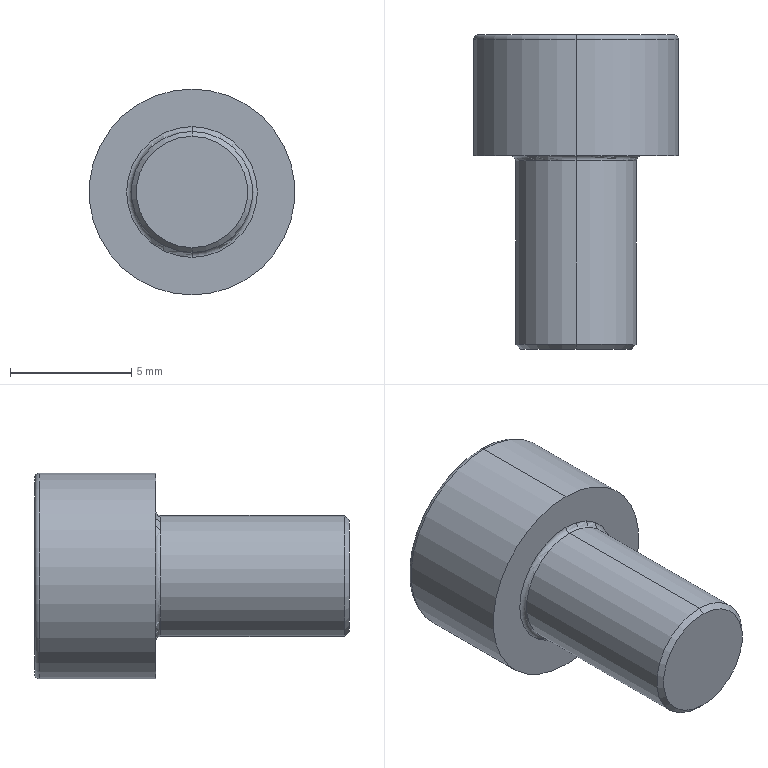Part | STEP file | 1 solid | 20 faces | box 8.5 x 13 x 8.5 mm | volume 405.768 mm3 | plane 10 | torus 4 | cylinder 4 | cone 2 | commonest cylinder face diameters 5 x2 8.5 x2
STEP:
#1=CARTESIAN_POINT('',(0.,-8.,-2.3));
#2=VERTEX_POINT('',#1);
#3=CARTESIAN_POINT('',(0.,-8.,2.3));
#4=VERTEX_POINT('',#3);
#5=CARTESIAN_POINT('',(0.,-8.,0.));
#6=DIRECTION('',(0.,-1.,0.));
#7=DIRECTION('',(0.,0.,-1.));
#8=AXIS2_PLACEMENT_3D('',#5,#6,#7);
#9=CIRCLE('',#8,2.3);
#10=EDGE_CURVE('',#2,#4,#9,.T.);
#11=ORIENTED_EDGE('',*,*,#10,.F.);
#12=CARTESIAN_POINT('',(0.,-7.8,-2.5));
#13=VERTEX_POINT('',#12);
#14=CARTESIAN_POINT('',(0.,-8.,-2.3));
#15=DIRECTION('',(0.,0.7071,-0.7071));
#16=VECTOR('',#15,1000.);
#17=LINE('',#14,#16);
#18=EDGE_CURVE('',#2,#13,#17,.T.);
#19=ORIENTED_EDGE('',*,*,#18,.T.);
#20=CARTESIAN_POINT('',(0.,-7.8,2.5));
#21=VERTEX_POINT('',#20);
#22=CARTESIAN_POINT('',(0.,-7.8,0.));
#23=DIRECTION('',(0.,1.,0.));
#24=DIRECTION('',(0.,0.,-1.));
#25=AXIS2_PLACEMENT_3D('',#22,#23,#24);
#26=CIRCLE('',#25,2.5);
#27=EDGE_CURVE('',#21,#13,#26,.T.);
#28=ORIENTED_EDGE('',*,*,#27,.F.);
#29=CARTESIAN_POINT('',(0.,-8.,2.3));
#30=DIRECTION('',(0.,0.7071,0.7071));
#31=VECTOR('',#30,1000.);
#32=LINE('',#29,#31);
#33=EDGE_CURVE('',#4,#21,#32,.T.);
#34=ORIENTED_EDGE('',*,*,#33,.F.);
#35=EDGE_LOOP('',(#11,#19,#28,#34));
#36=FACE_OUTER_BOUND('',#35,.T.);
#37=CARTESIAN_POINT('',(0.,-8.,0.));
#38=DIRECTION('',(0.,1.,0.));
#39=DIRECTION('',(0.,0.,1.));
#40=AXIS2_PLACEMENT_3D('',#37,#38,#39);
#41=CONICAL_SURFACE('',#40,2.3,0.7854);
#42=ADVANCED_FACE('',(#36),#41,.T.);
#43=CARTESIAN_POINT('',(0.,4.8,-4.25));
#44=VERTEX_POINT('',#43);
#45=CARTESIAN_POINT('',(0.,4.8,4.25));
#46=VERTEX_POINT('',#45);
#47=CARTESIAN_POINT('',(0.,4.8,0.));
#48=DIRECTION('',(0.,-1.,0.));
#49=DIRECTION('',(0.,0.,1.));
#50=AXIS2_PLACEMENT_3D('',#47,#48,#49);
#51=CIRCLE('',#50,4.25);
#52=EDGE_CURVE('',#44,#46,#51,.T.);
#53=ORIENTED_EDGE('',*,*,#52,.F.);
#54=CARTESIAN_POINT('',(0.,5.,-4.05));
#55=VERTEX_POINT('',#54);
#56=CARTESIAN_POINT('',(0.,4.8,-4.05));
#57=DIRECTION('',(1.,0.,0.));
#58=DIRECTION('',(0.,0.,-1.));
#59=AXIS2_PLACEMENT_3D('',#56,#57,#58);
#60=CIRCLE('',#59,0.2);
#61=EDGE_CURVE('',#44,#55,#60,.T.);
#62=ORIENTED_EDGE('',*,*,#61,.T.);
#63=CARTESIAN_POINT('',(0.,5.,4.05));
#64=VERTEX_POINT('',#63);
#65=CARTESIAN_POINT('',(0.,5.,0.));
#66=DIRECTION('',(0.,1.,0.));
#67=DIRECTION('',(0.,0.,1.));
#68=AXIS2_PLACEMENT_3D('',#65,#66,#67);
#69=CIRCLE('',#68,4.05);
#70=EDGE_CURVE('',#64,#55,#69,.T.);
#71=ORIENTED_EDGE('',*,*,#70,.F.);
#72=CARTESIAN_POINT('',(0.,4.8,4.05));
#73=DIRECTION('',(-1.,0.,0.));
#74=DIRECTION('',(0.,0.,1.));
#75=AXIS2_PLACEMENT_3D('',#72,#73,#74);
#76=CIRCLE('',#75,0.2);
#77=EDGE_CURVE('',#46,#64,#76,.T.);
#78=ORIENTED_EDGE('',*,*,#77,.F.);
#79=EDGE_LOOP('',(#53,#62,#71,#78));
#80=FACE_OUTER_BOUND('',#79,.T.);
#81=CARTESIAN_POINT('',(0.,4.8,0.));
#82=DIRECTION('',(0.,1.,0.));
#83=DIRECTION('',(0.,0.,1.));
#84=AXIS2_PLACEMENT_3D('',#81,#82,#83);
#85=TOROIDAL_SURFACE('',#84,4.05,0.2);
#86=ADVANCED_FACE('',(#80),#85,.T.);
#87=CARTESIAN_POINT('',(0.,-0.2,2.5));
#88=VERTEX_POINT('',#87);
#89=CARTESIAN_POINT('',(0.,-0.2,-2.5));
#90=VERTEX_POINT('',#89);
#91=CARTESIAN_POINT('',(0.,-0.2,0.));
#92=DIRECTION('',(0.,-1.,0.));
#93=DIRECTION('',(0.,0.,-1.));
#94=AXIS2_PLACEMENT_3D('',#91,#92,#93);
#95=CIRCLE('',#94,2.5);
#96=EDGE_CURVE('',#88,#90,#95,.T.);
#97=ORIENTED_EDGE('',*,*,#96,.F.);
#98=CARTESIAN_POINT('',(0.,0.,2.7));
#99=VERTEX_POINT('',#98);
#100=CARTESIAN_POINT('',(0.,-0.2,2.7));
#101=DIRECTION('',(1.,0.,0.));
#102=DIRECTION('',(0.,0.,-1.));
#103=AXIS2_PLACEMENT_3D('',#100,#101,#102);
#104=CIRCLE('',#103,0.2);
#105=EDGE_CURVE('',#88,#99,#104,.T.);
#106=ORIENTED_EDGE('',*,*,#105,.T.);
#107=CARTESIAN_POINT('',(0.,0.,-2.7));
#108=VERTEX_POINT('',#107);
#109=CARTESIAN_POINT('',(0.,0.,0.));
#110=DIRECTION('',(0.,1.,0.));
#111=DIRECTION('',(0.,0.,-1.));
#112=AXIS2_PLACEMENT_3D('',#109,#110,#111);
#113=CIRCLE('',#112,2.7);
#114=EDGE_CURVE('',#108,#99,#113,.T.);
#115=ORIENTED_EDGE('',*,*,#114,.F.);
#116=CARTESIAN_POINT('',(0.,-0.2,-2.7));
#117=DIRECTION('',(-1.,0.,0.));
#118=DIRECTION('',(0.,0.,1.));
#119=AXIS2_PLACEMENT_3D('',#116,#117,#118);
#120=CIRCLE('',#119,0.2);
#121=EDGE_CURVE('',#90,#108,#120,.T.);
#122=ORIENTED_EDGE('',*,*,#121,.F.);
#123=EDGE_LOOP('',(#97,#106,#115,#122));
#124=FACE_OUTER_BOUND('',#123,.T.);
#125=CARTESIAN_POINT('',(0.,-0.2,0.));
#126=DIRECTION('',(0.,-1.,0.));
#127=DIRECTION('',(0.,0.,-1.));
#128=AXIS2_PLACEMENT_3D('',#125,#126,#127);
#129=TOROIDAL_SURFACE('',#128,2.7,0.2);
#130=ADVANCED_FACE('',(#124),#129,.F.);
#131=CARTESIAN_POINT('',(0.,-0.2,0.));
#132=DIRECTION('',(0.,-1.,0.));
#133=DIRECTION('',(0.,0.,-1.));
#134=AXIS2_PLACEMENT_3D('',#131,#132,#133);
#135=CIRCLE('',#134,2.5);
#136=EDGE_CURVE('',#90,#88,#135,.T.);
#137=ORIENTED_EDGE('',*,*,#136,.T.);
#138=CARTESIAN_POINT('',(0.,0.,2.5));
#139=DIRECTION('',(0.,-1.,0.));
#140=VECTOR('',#139,1000.);
#141=LINE('',#138,#140);
#142=EDGE_CURVE('',#88,#21,#141,.T.);
#143=ORIENTED_EDGE('',*,*,#142,.T.);
#144=ORIENTED_EDGE('',*,*,#27,.T.);
#145=CARTESIAN_POINT('',(0.,0.,-2.5));
#146=DIRECTION('',(0.,-1.,0.));
#147=VECTOR('',#146,1000.);
#148=LINE('',#145,#147);
#149=EDGE_CURVE('',#90,#13,#148,.T.);
#150=ORIENTED_EDGE('',*,*,#149,.F.);
#151=EDGE_LOOP('',(#137,#143,#144,#150));
#152=FACE_OUTER_BOUND('',#151,.T.);
#153=CARTESIAN_POINT('',(0.,0.,0.));
#154=DIRECTION('',(0.,-1.,0.));
#155=DIRECTION('',(0.,0.,-1.));
#156=AXIS2_PLACEMENT_3D('',#153,#154,#155);
#157=CYLINDRICAL_SURFACE('',#156,2.5);
#158=ADVANCED_FACE('',(#152),#157,.T.);
#159=ORIENTED_EDGE('',*,*,#52,.T.);
#160=CARTESIAN_POINT('',(0.,0.,4.25));
#161=VERTEX_POINT('',#160);
#162=CARTESIAN_POINT('',(0.,0.,4.25));
#163=DIRECTION('',(0.,-1.,0.));
#164=VECTOR('',#163,1000.);
#165=LINE('',#162,#164);
#166=EDGE_CURVE('',#46,#161,#165,.T.);
#167=ORIENTED_EDGE('',*,*,#166,.T.);
#168=CARTESIAN_POINT('',(0.,0.,-4.25));
#169=VERTEX_POINT('',#168);
#170=CARTESIAN_POINT('',(0.,0.,0.));
#171=DIRECTION('',(0.,-1.,0.));
#172=DIRECTION('',(0.,0.,-1.));
#173=AXIS2_PLACEMENT_3D('',#170,#171,#172);
#174=CIRCLE('',#173,4.25);
#175=EDGE_CURVE('',#169,#161,#174,.T.);
#176=ORIENTED_EDGE('',*,*,#175,.F.);
#177=CARTESIAN_POINT('',(0.,0.,-4.25));
#178=DIRECTION('',(0.,-1.,0.));
#179=VECTOR('',#178,1000.);
#180=LINE('',#177,#179);
#181=EDGE_CURVE('',#44,#169,#180,.T.);
#182=ORIENTED_EDGE('',*,*,#181,.F.);
#183=EDGE_LOOP('',(#159,#167,#176,#182));
#184=FACE_OUTER_BOUND('',#183,.T.);
#185=CARTESIAN_POINT('',(0.,0.,0.));
#186=DIRECTION('',(0.,-1.,0.));
#187=DIRECTION('',(0.,0.,-1.));
#188=AXIS2_PLACEMENT_3D('',#185,#186,#187);
#189=CYLINDRICAL_SURFACE('',#188,4.25);
#190=ADVANCED_FACE('',(#184),#189,.T.);
#191=ORIENTED_EDGE('',*,*,#70,.T.);
#192=CARTESIAN_POINT('',(0.,5.,0.));
#193=DIRECTION('',(0.,1.,0.));
#194=DIRECTION('',(0.,0.,1.));
#195=AXIS2_PLACEMENT_3D('',#192,#193,#194);
#196=CIRCLE('',#195,4.05);
#197=EDGE_CURVE('',#55,#64,#196,.T.);
#198=ORIENTED_EDGE('',*,*,#197,.T.);
#199=EDGE_LOOP('',(#191,#198));
#200=FACE_OUTER_BOUND('',#199,.T.);
#201=CARTESIAN_POINT('',(0.,5.,-2.309));
#202=VERTEX_POINT('',#201);
#203=CARTESIAN_POINT('',(-2.,5.,-1.155));
#204=VERTEX_POINT('',#203);
#205=CARTESIAN_POINT('',(0.,5.,-2.309));
#206=DIRECTION('',(-0.866,0.,0.5));
#207=VECTOR('',#206,1000.);
#208=LINE('',#205,#207);
#209=EDGE_CURVE('',#202,#204,#208,.T.);
#210=ORIENTED_EDGE('',*,*,#209,.F.);
#211=CARTESIAN_POINT('',(2.,5.,-1.155));
#212=VERTEX_POINT('',#211);
#213=CARTESIAN_POINT('',(2.,5.,-1.155));
#214=DIRECTION('',(-0.866,0.,-0.5));
#215=VECTOR('',#214,1000.);
#216=LINE('',#213,#215);
#217=EDGE_CURVE('',#212,#202,#216,.T.);
#218=ORIENTED_EDGE('',*,*,#217,.F.);
#219=CARTESIAN_POINT('',(2.,5.,1.155));
#220=VERTEX_POINT('',#219);
#221=CARTESIAN_POINT('',(2.,5.,1.155));
#222=DIRECTION('',(0.,0.,-1.));
#223=VECTOR('',#222,1000.);
#224=LINE('',#221,#223);
#225=EDGE_CURVE('',#220,#212,#224,.T.);
#226=ORIENTED_EDGE('',*,*,#225,.F.);
#227=CARTESIAN_POINT('',(0.,5.,2.309));
#228=VERTEX_POINT('',#227);
#229=CARTESIAN_POINT('',(0.,5.,2.309));
#230=DIRECTION('',(0.866,0.,-0.5));
#231=VECTOR('',#230,1000.);
#232=LINE('',#229,#231);
#233=EDGE_CURVE('',#228,#220,#232,.T.);
#234=ORIENTED_EDGE('',*,*,#233,.F.);
#235=CARTESIAN_POINT('',(-2.,5.,1.155));
#236=VERTEX_POINT('',#235);
#237=CARTESIAN_POINT('',(-2.,5.,1.155));
#238=DIRECTION('',(0.866,0.,0.5));
#239=VECTOR('',#238,1000.);
#240=LINE('',#237,#239);
#241=EDGE_CURVE('',#236,#228,#240,.T.);
#242=ORIENTED_EDGE('',*,*,#241,.F.);
#243=CARTESIAN_POINT('',(-2.,5.,-1.155));
#244=DIRECTION('',(0.,0.,1.));
#245=VECTOR('',#244,1000.);
#246=LINE('',#243,#245);
#247=EDGE_CURVE('',#204,#236,#246,.T.);
#248=ORIENTED_EDGE('',*,*,#247,.F.);
#249=EDGE_LOOP('',(#210,#218,#226,#234,#242,#248));
#250=FACE_BOUND('',#249,.T.);
#251=CARTESIAN_POINT('',(0.,5.,0.));
#252=DIRECTION('',(0.,1.,0.));
#253=DIRECTION('',(0.,0.,1.));
#254=AXIS2_PLACEMENT_3D('',#251,#252,#253);
#255=PLANE('',#254);
#256=ADVANCED_FACE('',(#200,#250),#255,.T.);
#257=ORIENTED_EDGE('',*,*,#166,.F.);
#258=CARTESIAN_POINT('',(0.,4.8,0.));
#259=DIRECTION('',(0.,-1.,0.));
#260=DIRECTION('',(0.,0.,1.));
#261=AXIS2_PLACEMENT_3D('',#258,#259,#260);
#262=CIRCLE('',#261,4.25);
#263=EDGE_CURVE('',#46,#44,#262,.T.);
#264=ORIENTED_EDGE('',*,*,#263,.T.);
#265=ORIENTED_EDGE('',*,*,#181,.T.);
#266=CARTESIAN_POINT('',(0.,0.,0.));
#267=DIRECTION('',(0.,-1.,0.));
#268=DIRECTION('',(0.,0.,-1.));
#269=AXIS2_PLACEMENT_3D('',#266,#267,#268);
#270=CIRCLE('',#269,4.25);
#271=EDGE_CURVE('',#161,#169,#270,.T.);
#272=ORIENTED_EDGE('',*,*,#271,.F.);
#273=EDGE_LOOP('',(#257,#264,#265,#272));
#274=FACE_OUTER_BOUND('',#273,.T.);
#275=CARTESIAN_POINT('',(0.,0.,0.));
#276=DIRECTION('',(0.,-1.,0.));
#277=DIRECTION('',(0.,0.,-1.));
#278=AXIS2_PLACEMENT_3D('',#275,#276,#277);
#279=CYLINDRICAL_SURFACE('',#278,4.25);
#280=ADVANCED_FACE('',(#274),#279,.T.);
#281=ORIENTED_EDGE('',*,*,#114,.T.);
#282=CARTESIAN_POINT('',(0.,0.,0.));
#283=DIRECTION('',(0.,1.,0.));
#284=DIRECTION('',(0.,0.,-1.));
#285=AXIS2_PLACEMENT_3D('',#282,#283,#284);
#286=CIRCLE('',#285,2.7);
#287=EDGE_CURVE('',#99,#108,#286,.T.);
#288=ORIENTED_EDGE('',*,*,#287,.T.);
#289=EDGE_LOOP('',(#281,#288));
#290=FACE_BOUND('',#289,.T.);
#291=ORIENTED_EDGE('',*,*,#175,.T.);
#292=ORIENTED_EDGE('',*,*,#271,.T.);
#293=EDGE_LOOP('',(#291,#292));
#294=FACE_OUTER_BOUND('',#293,.T.);
#295=CARTESIAN_POINT('',(4.25,0.,0.));
#296=DIRECTION('',(0.,-1.,0.));
#297=DIRECTION('',(0.,0.,-1.));
#298=AXIS2_PLACEMENT_3D('',#295,#296,#297);
#299=PLANE('',#298);
#300=ADVANCED_FACE('',(#290,#294),#299,.T.);
#301=ORIENTED_EDGE('',*,*,#142,.F.);
#302=ORIENTED_EDGE('',*,*,#96,.T.);
#303=ORIENTED_EDGE('',*,*,#149,.T.);
#304=CARTESIAN_POINT('',(0.,-7.8,0.));
#305=DIRECTION('',(0.,1.,0.));
#306=DIRECTION('',(0.,0.,-1.));
#307=AXIS2_PLACEMENT_3D('',#304,#305,#306);
#308=CIRCLE('',#307,2.5);
#309=EDGE_CURVE('',#13,#21,#308,.T.);
#310=ORIENTED_EDGE('',*,*,#309,.T.);
#311=EDGE_LOOP('',(#301,#302,#303,#310));
#312=FACE_OUTER_BOUND('',#311,.T.);
#313=CARTESIAN_POINT('',(0.,0.,0.));
#314=DIRECTION('',(0.,-1.,0.));
#315=DIRECTION('',(0.,0.,-1.));
#316=AXIS2_PLACEMENT_3D('',#313,#314,#315);
#317=CYLINDRICAL_SURFACE('',#316,2.5);
#318=ADVANCED_FACE('',(#312),#317,.T.);
#319=CARTESIAN_POINT('',(0.,-8.,0.));
#320=DIRECTION('',(0.,-1.,0.));
#321=DIRECTION('',(0.,0.,-1.));
#322=AXIS2_PLACEMENT_3D('',#319,#320,#321);
#323=CIRCLE('',#322,2.3);
#324=EDGE_CURVE('',#4,#2,#323,.T.);
#325=ORIENTED_EDGE('',*,*,#324,.T.);
#326=ORIENTED_EDGE('',*,*,#10,.T.);
#327=EDGE_LOOP('',(#325,#326));
#328=FACE_OUTER_BOUND('',#327,.T.);
#329=CARTESIAN_POINT('',(2.5,-8.,0.));
#330=DIRECTION('',(0.,-1.,0.));
#331=DIRECTION('',(0.,0.,-1.));
#332=AXIS2_PLACEMENT_3D('',#329,#330,#331);
#333=PLANE('',#332);
#334=ADVANCED_FACE('',(#328),#333,.T.);
#335=ORIENTED_EDGE('',*,*,#209,.T.);
#336=CARTESIAN_POINT('',(-2.,2.5,-1.155));
#337=VERTEX_POINT('',#336);
#338=CARTESIAN_POINT('',(-2.,2.5,-1.155));
#339=DIRECTION('',(0.,1.,0.));
#340=VECTOR('',#339,1000.);
#341=LINE('',#338,#340);
#342=EDGE_CURVE('',#337,#204,#341,.T.);
#343=ORIENTED_EDGE('',*,*,#342,.F.);
#344=CARTESIAN_POINT('',(0.,2.5,-2.309));
#345=VERTEX_POINT('',#344);
#346=CARTESIAN_POINT('',(0.,2.5,-2.309));
#347=DIRECTION('',(-0.866,0.,0.5));
#348=VECTOR('',#347,1000.);
#349=LINE('',#346,#348);
#350=EDGE_CURVE('',#345,#337,#349,.T.);
#351=ORIENTED_EDGE('',*,*,#350,.F.);
#352=CARTESIAN_POINT('',(0.,2.5,-2.309));
#353=DIRECTION('',(0.,1.,0.));
#354=VECTOR('',#353,1000.);
#355=LINE('',#352,#354);
#356=EDGE_CURVE('',#345,#202,#355,.T.);
#357=ORIENTED_EDGE('',*,*,#356,.T.);
#358=EDGE_LOOP('',(#335,#343,#351,#357));
#359=FACE_OUTER_BOUND('',#358,.T.);
#360=CARTESIAN_POINT('',(0.,2.5,-2.309));
#361=DIRECTION('',(-0.5,0.,-0.866));
#362=DIRECTION('',(-0.866,0.,0.5));
#363=AXIS2_PLACEMENT_3D('',#360,#361,#362);
#364=PLANE('',#363);
#365=ADVANCED_FACE('',(#359),#364,.F.);
#366=ORIENTED_EDGE('',*,*,#217,.T.);
#367=ORIENTED_EDGE('',*,*,#356,.F.);
#368=CARTESIAN_POINT('',(2.,2.5,-1.155));
#369=VERTEX_POINT('',#368);
#370=CARTESIAN_POINT('',(2.,2.5,-1.155));
#371=DIRECTION('',(-0.866,0.,-0.5));
#372=VECTOR('',#371,1000.);
#373=LINE('',#370,#372);
#374=EDGE_CURVE('',#369,#345,#373,.T.);
#375=ORIENTED_EDGE('',*,*,#374,.F.);
#376=CARTESIAN_POINT('',(2.,2.5,-1.155));
#377=DIRECTION('',(0.,1.,0.));
#378=VECTOR('',#377,1000.);
#379=LINE('',#376,#378);
#380=EDGE_CURVE('',#369,#212,#379,.T.);
#381=ORIENTED_EDGE('',*,*,#380,.T.);
#382=EDGE_LOOP('',(#366,#367,#375,#381));
#383=FACE_OUTER_BOUND('',#382,.T.);
#384=CARTESIAN_POINT('',(2.,2.5,-1.155));
#385=DIRECTION('',(0.5,0.,-0.866));
#386=DIRECTION('',(-0.866,0.,-0.5));
#387=AXIS2_PLACEMENT_3D('',#384,#385,#386);
#388=PLANE('',#387);
#389=ADVANCED_FACE('',(#383),#388,.F.);
#390=ORIENTED_EDGE('',*,*,#225,.T.);
#391=ORIENTED_EDGE('',*,*,#380,.F.);
#392=CARTESIAN_POINT('',(2.,2.5,1.155));
#393=VERTEX_POINT('',#392);
#394=CARTESIAN_POINT('',(2.,2.5,1.155));
#395=DIRECTION('',(0.,0.,-1.));
#396=VECTOR('',#395,1000.);
#397=LINE('',#394,#396);
#398=EDGE_CURVE('',#393,#369,#397,.T.);
#399=ORIENTED_EDGE('',*,*,#398,.F.);
#400=CARTESIAN_POINT('',(2.,2.5,1.155));
#401=DIRECTION('',(0.,1.,0.));
#402=VECTOR('',#401,1000.);
#403=LINE('',#400,#402);
#404=EDGE_CURVE('',#393,#220,#403,.T.);
#405=ORIENTED_EDGE('',*,*,#404,.T.);
#406=EDGE_LOOP('',(#390,#391,#399,#405));
#407=FACE_OUTER_BOUND('',#406,.T.);
#408=CARTESIAN_POINT('',(2.,2.5,1.155));
#409=DIRECTION('',(1.,0.,0.));
#410=DIRECTION('',(0.,0.,-1.));
#411=AXIS2_PLACEMENT_3D('',#408,#409,#410);
#412=PLANE('',#411);
#413=ADVANCED_FACE('',(#407),#412,.F.);
#414=ORIENTED_EDGE('',*,*,#233,.T.);
#415=ORIENTED_EDGE('',*,*,#404,.F.);
#416=CARTESIAN_POINT('',(0.,2.5,2.309));
#417=VERTEX_POINT('',#416);
#418=CARTESIAN_POINT('',(0.,2.5,2.309));
#419=DIRECTION('',(0.866,0.,-0.5));
#420=VECTOR('',#419,1000.);
#421=LINE('',#418,#420);
#422=EDGE_CURVE('',#417,#393,#421,.T.);
#423=ORIENTED_EDGE('',*,*,#422,.F.);
#424=CARTESIAN_POINT('',(0.,2.5,2.309));
#425=DIRECTION('',(0.,1.,0.));
#426=VECTOR('',#425,1000.);
#427=LINE('',#424,#426);
#428=EDGE_CURVE('',#417,#228,#427,.T.);
#429=ORIENTED_EDGE('',*,*,#428,.T.);
#430=EDGE_LOOP('',(#414,#415,#423,#429));
#431=FACE_OUTER_BOUND('',#430,.T.);
#432=CARTESIAN_POINT('',(0.,2.5,2.309));
#433=DIRECTION('',(0.5,0.,0.866));
#434=DIRECTION('',(0.866,0.,-0.5));
#435=AXIS2_PLACEMENT_3D('',#432,#433,#434);
#436=PLANE('',#435);
#437=ADVANCED_FACE('',(#431),#436,.F.);
#438=ORIENTED_EDGE('',*,*,#241,.T.);
#439=ORIENTED_EDGE('',*,*,#428,.F.);
#440=CARTESIAN_POINT('',(-2.,2.5,1.155));
#441=VERTEX_POINT('',#440);
#442=CARTESIAN_POINT('',(-2.,2.5,1.155));
#443=DIRECTION('',(0.866,0.,0.5));
#444=VECTOR('',#443,1000.);
#445=LINE('',#442,#444);
#446=EDGE_CURVE('',#441,#417,#445,.T.);
#447=ORIENTED_EDGE('',*,*,#446,.F.);
#448=CARTESIAN_POINT('',(-2.,2.5,1.155));
#449=DIRECTION('',(0.,1.,0.));
#450=VECTOR('',#449,1000.);
#451=LINE('',#448,#450);
#452=EDGE_CURVE('',#441,#236,#451,.T.);
#453=ORIENTED_EDGE('',*,*,#452,.T.);
#454=EDGE_LOOP('',(#438,#439,#447,#453));
#455=FACE_OUTER_BOUND('',#454,.T.);
#456=CARTESIAN_POINT('',(-2.,2.5,1.155));
#457=DIRECTION('',(-0.5,0.,0.866));
#458=DIRECTION('',(0.866,0.,0.5));
#459=AXIS2_PLACEMENT_3D('',#456,#457,#458);
#460=PLANE('',#459);
#461=ADVANCED_FACE('',(#455),#460,.F.);
#462=ORIENTED_EDGE('',*,*,#247,.T.);
#463=ORIENTED_EDGE('',*,*,#452,.F.);
#464=CARTESIAN_POINT('',(-2.,2.5,-1.155));
#465=DIRECTION('',(0.,0.,1.));
#466=VECTOR('',#465,1000.);
#467=LINE('',#464,#466);
#468=EDGE_CURVE('',#337,#441,#467,.T.);
#469=ORIENTED_EDGE('',*,*,#468,.F.);
#470=ORIENTED_EDGE('',*,*,#342,.T.);
#471=EDGE_LOOP('',(#462,#463,#469,#470));
#472=FACE_OUTER_BOUND('',#471,.T.);
#473=CARTESIAN_POINT('',(-2.,2.5,-1.155));
#474=DIRECTION('',(-1.,0.,0.));
#475=DIRECTION('',(0.,0.,1.));
#476=AXIS2_PLACEMENT_3D('',#473,#474,#475);
#477=PLANE('',#476);
#478=ADVANCED_FACE('',(#472),#477,.F.);
#479=ORIENTED_EDGE('',*,*,#350,.T.);
#480=ORIENTED_EDGE('',*,*,#468,.T.);
#481=ORIENTED_EDGE('',*,*,#446,.T.);
#482=ORIENTED_EDGE('',*,*,#422,.T.);
#483=ORIENTED_EDGE('',*,*,#398,.T.);
#484=ORIENTED_EDGE('',*,*,#374,.T.);
#485=EDGE_LOOP('',(#479,#480,#481,#482,#483,#484));
#486=FACE_OUTER_BOUND('',#485,.T.);
#487=CARTESIAN_POINT('',(0.,2.5,0.));
#488=DIRECTION('',(0.,1.,0.));
#489=DIRECTION('',(0.,0.,1.));
#490=AXIS2_PLACEMENT_3D('',#487,#488,#489);
#491=PLANE('',#490);
#492=ADVANCED_FACE('',(#486),#491,.T.);
#493=ORIENTED_EDGE('',*,*,#105,.F.);
#494=ORIENTED_EDGE('',*,*,#136,.F.);
#495=ORIENTED_EDGE('',*,*,#121,.T.);
#496=ORIENTED_EDGE('',*,*,#287,.F.);
#497=EDGE_LOOP('',(#493,#494,#495,#496));
#498=FACE_OUTER_BOUND('',#497,.T.);
#499=CARTESIAN_POINT('',(0.,-0.2,0.));
#500=DIRECTION('',(0.,-1.,0.));
#501=DIRECTION('',(0.,0.,-1.));
#502=AXIS2_PLACEMENT_3D('',#499,#500,#501);
#503=TOROIDAL_SURFACE('',#502,2.7,0.2);
#504=ADVANCED_FACE('',(#498),#503,.F.);
#505=ORIENTED_EDGE('',*,*,#61,.F.);
#506=ORIENTED_EDGE('',*,*,#263,.F.);
#507=ORIENTED_EDGE('',*,*,#77,.T.);
#508=ORIENTED_EDGE('',*,*,#197,.F.);
#509=EDGE_LOOP('',(#505,#506,#507,#508));
#510=FACE_OUTER_BOUND('',#509,.T.);
#511=CARTESIAN_POINT('',(0.,4.8,0.));
#512=DIRECTION('',(0.,1.,0.));
#513=DIRECTION('',(0.,0.,1.));
#514=AXIS2_PLACEMENT_3D('',#511,#512,#513);
#515=TOROIDAL_SURFACE('',#514,4.05,0.2);
#516=ADVANCED_FACE('',(#510),#515,.T.);
#517=ORIENTED_EDGE('',*,*,#18,.F.);
#518=ORIENTED_EDGE('',*,*,#324,.F.);
#519=ORIENTED_EDGE('',*,*,#33,.T.);
#520=ORIENTED_EDGE('',*,*,#309,.F.);
#521=EDGE_LOOP('',(#517,#518,#519,#520));
#522=FACE_OUTER_BOUND('',#521,.T.);
#523=CARTESIAN_POINT('',(0.,-8.,0.));
#524=DIRECTION('',(0.,1.,0.));
#525=DIRECTION('',(0.,0.,1.));
#526=AXIS2_PLACEMENT_3D('',#523,#524,#525);
#527=CONICAL_SURFACE('',#526,2.3,0.7854);
#528=ADVANCED_FACE('',(#522),#527,.T.);
#529=CLOSED_SHELL('',(#42,#86,#130,#158,#190,#256,#280,#300,#318,#334,#365,#389,#413,#437,#461,#478,#492,#504,#516,#528));
#530=MANIFOLD_SOLID_BREP('',#529);
#531=CARTESIAN_POINT('',(0.,0.,0.));
#532=DIRECTION('',(0.,0.,1.));
#533=DIRECTION('',(1.,0.,0.));
#534=AXIS2_PLACEMENT_3D('',#531,#532,#533);
#535=(LENGTH_UNIT()NAMED_UNIT(*)SI_UNIT(.MILLI.,.METRE.));
#536=UNCERTAINTY_MEASURE_WITH_UNIT(LENGTH_MEASURE(0.00001),#535,'','');
#537=(NAMED_UNIT(*)PLANE_ANGLE_UNIT()SI_UNIT($,.RADIAN.));
#538=(NAMED_UNIT(*)SI_UNIT($,.STERADIAN.)SOLID_ANGLE_UNIT());
#539=(GEOMETRIC_REPRESENTATION_CONTEXT(3)GLOBAL_UNCERTAINTY_ASSIGNED_CONTEXT((#536))GLOBAL_UNIT_ASSIGNED_CONTEXT((#535,#537,#538))REPRESENTATION_CONTEXT('',''));
#540=ADVANCED_BREP_SHAPE_REPRESENTATION('',(#530,#534),#539);